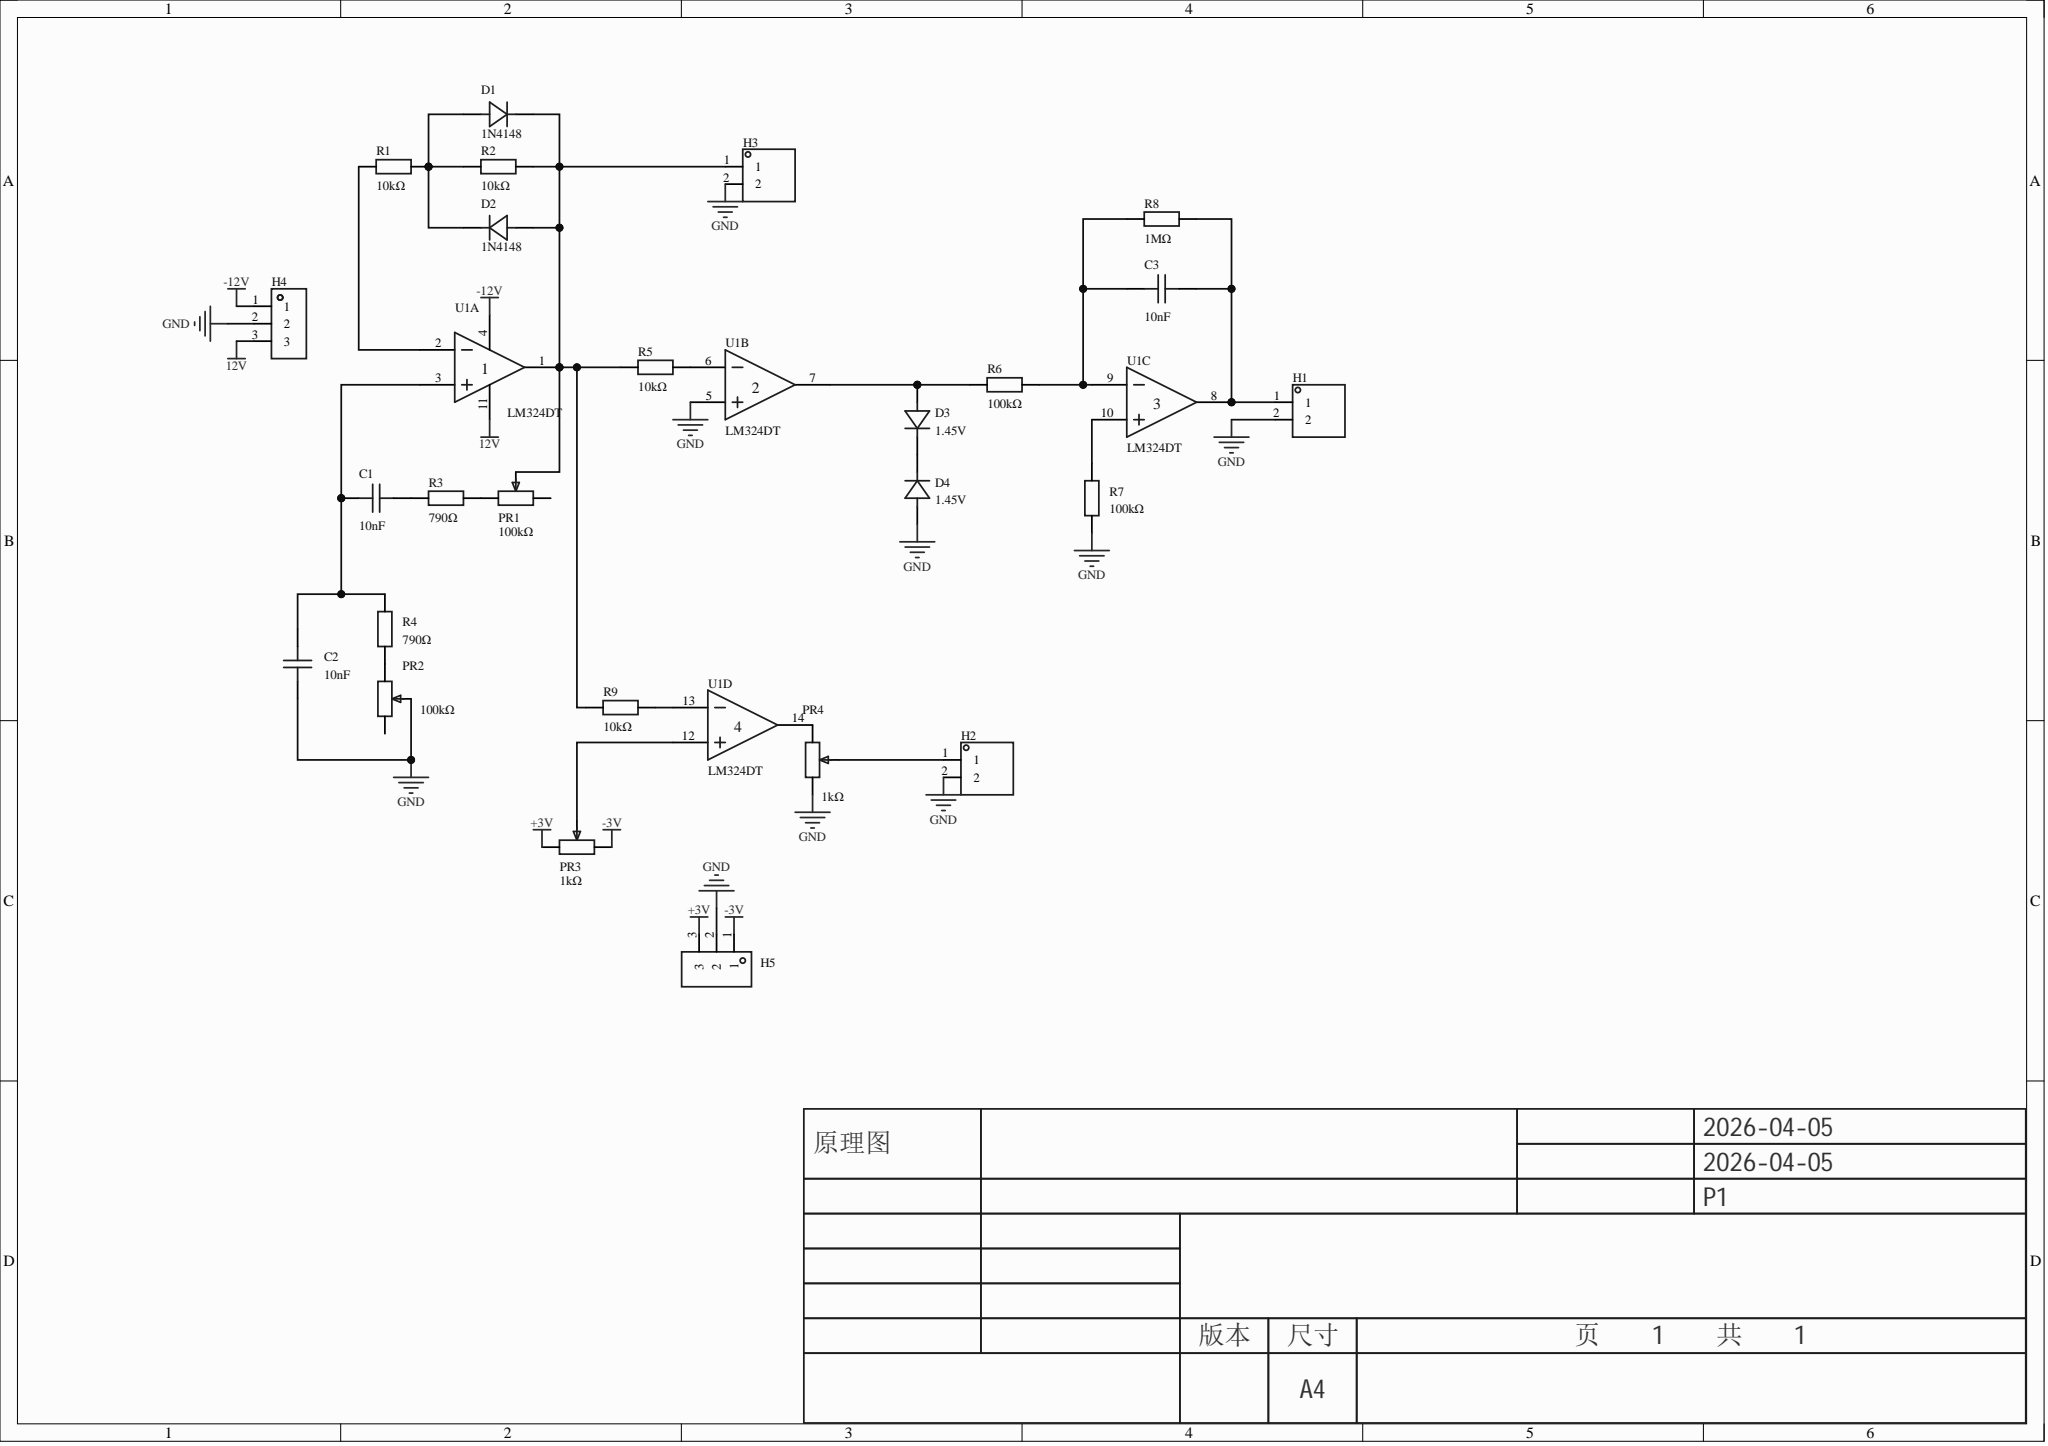Circuit board | Altium Designer | 26 parts | 22 nets
Bill of materials:
Comment,Description,Designator,Footprint,LibRef,Quantity
"10nF","","C1, C2, C3","CAP-TH_L7.2-W3.5-P5.00-D0.6","BFC237051103","3"
"1N4148","","D1, D2","DO-35_BD2.2-L4.0-D0.50_1N4148","1N4148_C18195411","2"
"1.45V","","D3, D4","DO-35_BD2.0-L4.2-P8.20-D0.5-RD","1SS54","2"
"","","H1, H2, H3","HDR-TH_2P-P2.54-V-M-1","HDR-M_2.54_1x2P","3"
"","","H4, H5","HDR-TH_3P-P2.54-V-M","HDR-M_2.54_1x3P","2"
"100kΩ","","PR1, PR2","R_3296","R_3296","2"
"1kΩ","","PR3, PR4","R_3296","R_3296","2"
"10kΩ","","R1, R2, R5, R9","Res_1/8W","Res_AXIAL-1/8W","4"
"790Ω","","R3, R4","Res_1/8W","Res_AXIAL-1/8W","2"
"100kΩ","","R6, R7","Res_1/8W","Res_AXIAL-1/8W","2"
"1MΩ","","R8","Res_1/8W","Res_AXIAL-1/8W","1"
"LM324DT","","U1","DIP-14_L19.2-W6.6-P2.54-LS10.9-BL","LM324DT","1"
Netlist (Protel format):
[
C1
CAP-TH_L7.2-W3.5-P5.00-D0.6
10nF



]
[
C2
CAP-TH_L7.2-W3.5-P5.00-D0.6
10nF



]
[
C3
CAP-TH_L7.2-W3.5-P5.00-D0.6
10nF



]
[
D1
DO-35_BD2.2-L4.0-D0.50_1N4148
1N4148



]
[
D2
DO-35_BD2.2-L4.0-D0.50_1N4148
1N4148



]
[
D3
DO-35_BD2.0-L4.2-P8.20-D0.5-RD
1.45V



]
[
D4
DO-35_BD2.0-L4.2-P8.20-D0.5-RD
1.45V



]
[
H1
HDR-TH_2P-P2.54-V-M-1




]
[
H2
HDR-TH_2P-P2.54-V-M-1




]
[
H3
HDR-TH_2P-P2.54-V-M-1




]
[
H4
HDR-TH_3P-P2.54-V-M




]
[
H5
HDR-TH_3P-P2.54-V-M




]
[
PR1
R_3296
100kΩ



]
[
PR2
R_3296
100kΩ



]
[
PR3
R_3296
1kΩ



]
[
PR4
R_3296
1kΩ



]
[
R1
Res_1/8W
10kΩ



]
[
R2
Res_1/8W
10kΩ



]
[
R3
Res_1/8W
790Ω



]
[
R4
Res_1/8W
790Ω



]
[
R5
Res_1/8W
10kΩ



]
[
R6
Res_1/8W
100kΩ



]
[
R7
Res_1/8W
100kΩ



]
[
R8
Res_1/8W
1MΩ



]
[
R9
Res_1/8W
10kΩ



]
[
U1
DIP-14_L19.2-W6.6-P2.54-LS10.9-BL
LM324DT



]
(
NetR9_2
R9-2
U1-13
)
(
NetR7_2
R7-2
U1-10
)
(
NetR5_2
R5-2
U1-6
)
(
NetR1_1
R1-1
U1-2
)
(
NetPR4_3
PR4-3
U1-14
)
(
NetPR3_2
PR3-2
U1-12
)
(
NetPR2_3
PR2-3
R4-2
)
(
NetPR1_3
PR1-3
R3-2
)
(
NetH2_1
H2-1
PR4-2
)
(
NetD3_2
D3-2
R6-1
U1-7
)
(
NetD3_1
D3-1
D4-1
)
(
NetD1_2
D1-2
D2-1
H3-1
PR1-2
R2-2
R5-1
R9-1
U1-1
)
(
NetD1_1
D1-1
D2-2
R1-2
R2-1
)
(
NetC3_2
C3-2
H1-1
R8-2
U1-8
)
(
NetC3_1
C3-1
R6-2
R8-1
U1-9
)
(
NetC1_2
C1-2
R3-1
)
(
NetC1_1
C1-1
C2-2
R4-1
U1-3
)
(
GND
C2-1
D4-2
H1-2
H2-2
H3-2
H4-2
H5-2
PR2-2
PR4-1
R7-1
U1-5
)
(
-12V
H4-1
U1-4
)
(
-3V
H5-1
PR3-1
)
(
+3V
H5-3
PR3-3
)
(
12V
H4-3
U1-11
)